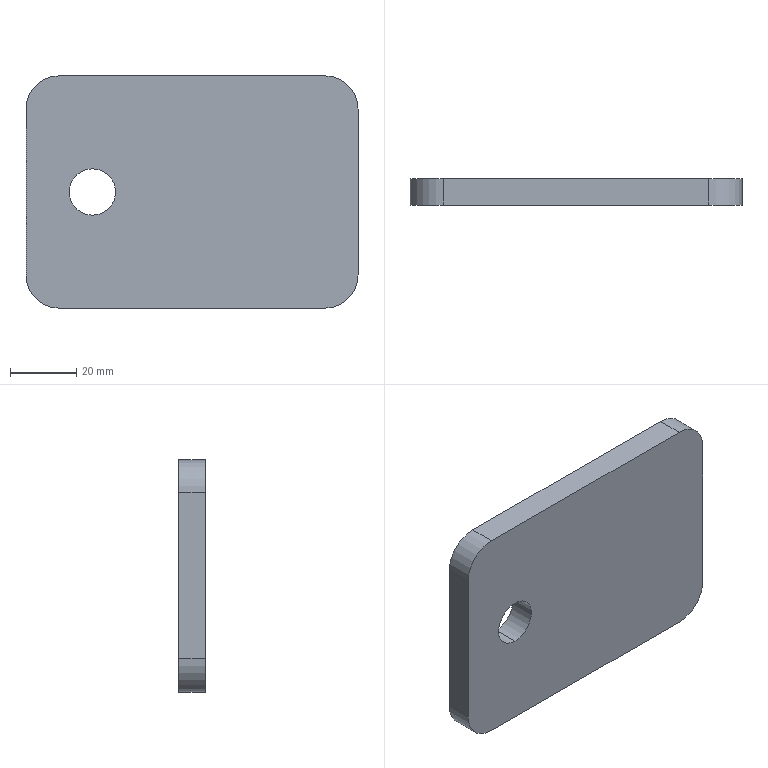Part | SolidWorks | features Extrusion 1, Fillet 1, ICE 1 | 1 solid | 12 faces | box 100 x 8 x 70 mm | volume 54082 mm3 | cylinder 6 | plane 6 | commonest cylinder face diameters 20 x4 14 x2
STEP:
#1=CARTESIAN_POINT('',(-30.,0.,-7.));
#2=VERTEX_POINT('',#1);
#3=CARTESIAN_POINT('',(-30.,0.,7.));
#4=VERTEX_POINT('',#3);
#5=CARTESIAN_POINT('',(-30.,0.,0.));
#6=DIRECTION('',(0.,1.,0.));
#7=DIRECTION('',(0.,0.,1.));
#8=AXIS2_PLACEMENT_3D('',#5,#6,#7);
#9=CIRCLE('',#8,7.);
#10=EDGE_CURVE('',#2,#4,#9,.T.);
#11=ORIENTED_EDGE('',*,*,#10,.F.);
#12=CARTESIAN_POINT('',(-30.,8.,-7.));
#13=VERTEX_POINT('',#12);
#14=CARTESIAN_POINT('',(-30.,0.,-7.));
#15=DIRECTION('',(0.,1.,0.));
#16=VECTOR('',#15,1000.);
#17=LINE('',#14,#16);
#18=EDGE_CURVE('',#2,#13,#17,.T.);
#19=ORIENTED_EDGE('',*,*,#18,.T.);
#20=CARTESIAN_POINT('',(-30.,8.,7.));
#21=VERTEX_POINT('',#20);
#22=CARTESIAN_POINT('',(-30.,8.,0.));
#23=DIRECTION('',(0.,1.,0.));
#24=DIRECTION('',(0.,0.,1.));
#25=AXIS2_PLACEMENT_3D('',#22,#23,#24);
#26=CIRCLE('',#25,7.);
#27=EDGE_CURVE('',#13,#21,#26,.T.);
#28=ORIENTED_EDGE('',*,*,#27,.T.);
#29=CARTESIAN_POINT('',(-30.,0.,7.));
#30=DIRECTION('',(0.,1.,0.));
#31=VECTOR('',#30,1000.);
#32=LINE('',#29,#31);
#33=EDGE_CURVE('',#4,#21,#32,.T.);
#34=ORIENTED_EDGE('',*,*,#33,.F.);
#35=EDGE_LOOP('',(#11,#19,#28,#34));
#36=FACE_OUTER_BOUND('',#35,.T.);
#37=CARTESIAN_POINT('',(-30.,0.,0.));
#38=DIRECTION('',(0.,1.,0.));
#39=DIRECTION('',(0.,0.,1.));
#40=AXIS2_PLACEMENT_3D('',#37,#38,#39);
#41=CYLINDRICAL_SURFACE('',#40,7.);
#42=ADVANCED_FACE('',(#36),#41,.F.);
#43=CARTESIAN_POINT('',(-50.,8.,-25.));
#44=VERTEX_POINT('',#43);
#45=CARTESIAN_POINT('',(-50.,8.,25.));
#46=VERTEX_POINT('',#45);
#47=CARTESIAN_POINT('',(-50.,8.,35.));
#48=DIRECTION('',(0.,0.,1.));
#49=VECTOR('',#48,1000.);
#50=LINE('',#47,#49);
#51=EDGE_CURVE('',#44,#46,#50,.T.);
#52=ORIENTED_EDGE('',*,*,#51,.F.);
#53=CARTESIAN_POINT('',(-50.,0.,-25.));
#54=VERTEX_POINT('',#53);
#55=CARTESIAN_POINT('',(-50.,8.,-25.));
#56=DIRECTION('',(0.,-1.,0.));
#57=VECTOR('',#56,1000.);
#58=LINE('',#55,#57);
#59=EDGE_CURVE('',#44,#54,#58,.T.);
#60=ORIENTED_EDGE('',*,*,#59,.T.);
#61=CARTESIAN_POINT('',(-50.,0.,25.));
#62=VERTEX_POINT('',#61);
#63=CARTESIAN_POINT('',(-50.,0.,35.));
#64=DIRECTION('',(0.,0.,1.));
#65=VECTOR('',#64,1000.);
#66=LINE('',#63,#65);
#67=EDGE_CURVE('',#54,#62,#66,.T.);
#68=ORIENTED_EDGE('',*,*,#67,.T.);
#69=CARTESIAN_POINT('',(-50.,8.,25.));
#70=DIRECTION('',(0.,1.,0.));
#71=VECTOR('',#70,1000.);
#72=LINE('',#69,#71);
#73=EDGE_CURVE('',#62,#46,#72,.T.);
#74=ORIENTED_EDGE('',*,*,#73,.T.);
#75=EDGE_LOOP('',(#52,#60,#68,#74));
#76=FACE_OUTER_BOUND('',#75,.T.);
#77=CARTESIAN_POINT('',(-50.,8.,35.));
#78=DIRECTION('',(1.,0.,0.));
#79=DIRECTION('',(0.,0.,-1.));
#80=AXIS2_PLACEMENT_3D('',#77,#78,#79);
#81=PLANE('',#80);
#82=ADVANCED_FACE('',(#76),#81,.F.);
#83=CARTESIAN_POINT('',(-40.,0.,35.));
#84=VERTEX_POINT('',#83);
#85=CARTESIAN_POINT('',(40.,0.,35.));
#86=VERTEX_POINT('',#85);
#87=CARTESIAN_POINT('',(50.,0.,35.));
#88=DIRECTION('',(1.,0.,0.));
#89=VECTOR('',#88,1000.);
#90=LINE('',#87,#89);
#91=EDGE_CURVE('',#84,#86,#90,.T.);
#92=ORIENTED_EDGE('',*,*,#91,.T.);
#93=CARTESIAN_POINT('',(40.,8.,35.));
#94=VERTEX_POINT('',#93);
#95=CARTESIAN_POINT('',(40.,8.,35.));
#96=DIRECTION('',(0.,1.,0.));
#97=VECTOR('',#96,1000.);
#98=LINE('',#95,#97);
#99=EDGE_CURVE('',#86,#94,#98,.T.);
#100=ORIENTED_EDGE('',*,*,#99,.T.);
#101=CARTESIAN_POINT('',(-40.,8.,35.));
#102=VERTEX_POINT('',#101);
#103=CARTESIAN_POINT('',(50.,8.,35.));
#104=DIRECTION('',(1.,0.,0.));
#105=VECTOR('',#104,1000.);
#106=LINE('',#103,#105);
#107=EDGE_CURVE('',#102,#94,#106,.T.);
#108=ORIENTED_EDGE('',*,*,#107,.F.);
#109=CARTESIAN_POINT('',(-40.,8.,35.));
#110=DIRECTION('',(0.,-1.,0.));
#111=VECTOR('',#110,1000.);
#112=LINE('',#109,#111);
#113=EDGE_CURVE('',#102,#84,#112,.T.);
#114=ORIENTED_EDGE('',*,*,#113,.T.);
#115=EDGE_LOOP('',(#92,#100,#108,#114));
#116=FACE_OUTER_BOUND('',#115,.T.);
#117=CARTESIAN_POINT('',(50.,8.,35.));
#118=DIRECTION('',(0.,0.,-1.));
#119=DIRECTION('',(-1.,0.,0.));
#120=AXIS2_PLACEMENT_3D('',#117,#118,#119);
#121=PLANE('',#120);
#122=ADVANCED_FACE('',(#116),#121,.F.);
#123=CARTESIAN_POINT('',(50.,0.,25.));
#124=VERTEX_POINT('',#123);
#125=CARTESIAN_POINT('',(50.,0.,-25.));
#126=VERTEX_POINT('',#125);
#127=CARTESIAN_POINT('',(50.,0.,35.));
#128=DIRECTION('',(0.,0.,-1.));
#129=VECTOR('',#128,1000.);
#130=LINE('',#127,#129);
#131=EDGE_CURVE('',#124,#126,#130,.T.);
#132=ORIENTED_EDGE('',*,*,#131,.T.);
#133=CARTESIAN_POINT('',(50.,8.,-25.));
#134=VERTEX_POINT('',#133);
#135=CARTESIAN_POINT('',(50.,8.,-25.));
#136=DIRECTION('',(0.,1.,0.));
#137=VECTOR('',#136,1000.);
#138=LINE('',#135,#137);
#139=EDGE_CURVE('',#126,#134,#138,.T.);
#140=ORIENTED_EDGE('',*,*,#139,.T.);
#141=CARTESIAN_POINT('',(50.,8.,25.));
#142=VERTEX_POINT('',#141);
#143=CARTESIAN_POINT('',(50.,8.,35.));
#144=DIRECTION('',(0.,0.,-1.));
#145=VECTOR('',#144,1000.);
#146=LINE('',#143,#145);
#147=EDGE_CURVE('',#142,#134,#146,.T.);
#148=ORIENTED_EDGE('',*,*,#147,.F.);
#149=CARTESIAN_POINT('',(50.,8.,25.));
#150=DIRECTION('',(0.,-1.,0.));
#151=VECTOR('',#150,1000.);
#152=LINE('',#149,#151);
#153=EDGE_CURVE('',#142,#124,#152,.T.);
#154=ORIENTED_EDGE('',*,*,#153,.T.);
#155=EDGE_LOOP('',(#132,#140,#148,#154));
#156=FACE_OUTER_BOUND('',#155,.T.);
#157=CARTESIAN_POINT('',(50.,8.,35.));
#158=DIRECTION('',(-1.,0.,0.));
#159=DIRECTION('',(0.,0.,1.));
#160=AXIS2_PLACEMENT_3D('',#157,#158,#159);
#161=PLANE('',#160);
#162=ADVANCED_FACE('',(#156),#161,.F.);
#163=CARTESIAN_POINT('',(40.,0.,-35.));
#164=VERTEX_POINT('',#163);
#165=CARTESIAN_POINT('',(-40.,0.,-35.));
#166=VERTEX_POINT('',#165);
#167=CARTESIAN_POINT('',(50.,0.,-35.));
#168=DIRECTION('',(-1.,0.,0.));
#169=VECTOR('',#168,1000.);
#170=LINE('',#167,#169);
#171=EDGE_CURVE('',#164,#166,#170,.T.);
#172=ORIENTED_EDGE('',*,*,#171,.T.);
#173=CARTESIAN_POINT('',(-40.,8.,-35.));
#174=VERTEX_POINT('',#173);
#175=CARTESIAN_POINT('',(-40.,8.,-35.));
#176=DIRECTION('',(0.,1.,0.));
#177=VECTOR('',#176,1000.);
#178=LINE('',#175,#177);
#179=EDGE_CURVE('',#166,#174,#178,.T.);
#180=ORIENTED_EDGE('',*,*,#179,.T.);
#181=CARTESIAN_POINT('',(40.,8.,-35.));
#182=VERTEX_POINT('',#181);
#183=CARTESIAN_POINT('',(50.,8.,-35.));
#184=DIRECTION('',(-1.,0.,0.));
#185=VECTOR('',#184,1000.);
#186=LINE('',#183,#185);
#187=EDGE_CURVE('',#182,#174,#186,.T.);
#188=ORIENTED_EDGE('',*,*,#187,.F.);
#189=CARTESIAN_POINT('',(40.,8.,-35.));
#190=DIRECTION('',(0.,-1.,0.));
#191=VECTOR('',#190,1000.);
#192=LINE('',#189,#191);
#193=EDGE_CURVE('',#182,#164,#192,.T.);
#194=ORIENTED_EDGE('',*,*,#193,.T.);
#195=EDGE_LOOP('',(#172,#180,#188,#194));
#196=FACE_OUTER_BOUND('',#195,.T.);
#197=CARTESIAN_POINT('',(50.,8.,-35.));
#198=DIRECTION('',(0.,0.,1.));
#199=DIRECTION('',(1.,0.,0.));
#200=AXIS2_PLACEMENT_3D('',#197,#198,#199);
#201=PLANE('',#200);
#202=ADVANCED_FACE('',(#196),#201,.F.);
#203=CARTESIAN_POINT('',(-30.,8.,0.));
#204=DIRECTION('',(0.,1.,0.));
#205=DIRECTION('',(0.,0.,1.));
#206=AXIS2_PLACEMENT_3D('',#203,#204,#205);
#207=CIRCLE('',#206,7.);
#208=EDGE_CURVE('',#21,#13,#207,.T.);
#209=ORIENTED_EDGE('',*,*,#208,.F.);
#210=ORIENTED_EDGE('',*,*,#27,.F.);
#211=EDGE_LOOP('',(#209,#210));
#212=FACE_BOUND('',#211,.T.);
#213=ORIENTED_EDGE('',*,*,#187,.T.);
#214=CARTESIAN_POINT('',(-40.,8.,-25.));
#215=DIRECTION('',(0.,1.,0.));
#216=DIRECTION('',(0.,0.,1.));
#217=AXIS2_PLACEMENT_3D('',#214,#215,#216);
#218=CIRCLE('',#217,10.);
#219=EDGE_CURVE('',#174,#44,#218,.T.);
#220=ORIENTED_EDGE('',*,*,#219,.T.);
#221=ORIENTED_EDGE('',*,*,#51,.T.);
#222=CARTESIAN_POINT('',(-40.,8.,25.));
#223=DIRECTION('',(0.,1.,0.));
#224=DIRECTION('',(0.,0.,1.));
#225=AXIS2_PLACEMENT_3D('',#222,#223,#224);
#226=CIRCLE('',#225,10.);
#227=EDGE_CURVE('',#46,#102,#226,.T.);
#228=ORIENTED_EDGE('',*,*,#227,.T.);
#229=ORIENTED_EDGE('',*,*,#107,.T.);
#230=CARTESIAN_POINT('',(40.,8.,25.));
#231=DIRECTION('',(0.,1.,0.));
#232=DIRECTION('',(0.,0.,1.));
#233=AXIS2_PLACEMENT_3D('',#230,#231,#232);
#234=CIRCLE('',#233,10.);
#235=EDGE_CURVE('',#94,#142,#234,.T.);
#236=ORIENTED_EDGE('',*,*,#235,.T.);
#237=ORIENTED_EDGE('',*,*,#147,.T.);
#238=CARTESIAN_POINT('',(40.,8.,-25.));
#239=DIRECTION('',(0.,1.,0.));
#240=DIRECTION('',(0.,0.,1.));
#241=AXIS2_PLACEMENT_3D('',#238,#239,#240);
#242=CIRCLE('',#241,10.);
#243=EDGE_CURVE('',#134,#182,#242,.T.);
#244=ORIENTED_EDGE('',*,*,#243,.T.);
#245=EDGE_LOOP('',(#213,#220,#221,#228,#229,#236,#237,#244));
#246=FACE_OUTER_BOUND('',#245,.T.);
#247=CARTESIAN_POINT('',(0.,8.,0.));
#248=DIRECTION('',(0.,1.,0.));
#249=DIRECTION('',(0.,0.,1.));
#250=AXIS2_PLACEMENT_3D('',#247,#248,#249);
#251=PLANE('',#250);
#252=ADVANCED_FACE('',(#212,#246),#251,.T.);
#253=CARTESIAN_POINT('',(-30.,0.,0.));
#254=DIRECTION('',(0.,1.,0.));
#255=DIRECTION('',(0.,0.,1.));
#256=AXIS2_PLACEMENT_3D('',#253,#254,#255);
#257=CIRCLE('',#256,7.);
#258=EDGE_CURVE('',#4,#2,#257,.T.);
#259=ORIENTED_EDGE('',*,*,#258,.T.);
#260=ORIENTED_EDGE('',*,*,#10,.T.);
#261=EDGE_LOOP('',(#259,#260));
#262=FACE_BOUND('',#261,.T.);
#263=ORIENTED_EDGE('',*,*,#67,.F.);
#264=CARTESIAN_POINT('',(-40.,0.,-25.));
#265=DIRECTION('',(0.,-1.,0.));
#266=DIRECTION('',(0.,0.,1.));
#267=AXIS2_PLACEMENT_3D('',#264,#265,#266);
#268=CIRCLE('',#267,10.);
#269=EDGE_CURVE('',#54,#166,#268,.T.);
#270=ORIENTED_EDGE('',*,*,#269,.T.);
#271=ORIENTED_EDGE('',*,*,#171,.F.);
#272=CARTESIAN_POINT('',(40.,0.,-25.));
#273=DIRECTION('',(0.,-1.,0.));
#274=DIRECTION('',(0.,0.,1.));
#275=AXIS2_PLACEMENT_3D('',#272,#273,#274);
#276=CIRCLE('',#275,10.);
#277=EDGE_CURVE('',#164,#126,#276,.T.);
#278=ORIENTED_EDGE('',*,*,#277,.T.);
#279=ORIENTED_EDGE('',*,*,#131,.F.);
#280=CARTESIAN_POINT('',(40.,0.,25.));
#281=DIRECTION('',(0.,-1.,0.));
#282=DIRECTION('',(0.,0.,1.));
#283=AXIS2_PLACEMENT_3D('',#280,#281,#282);
#284=CIRCLE('',#283,10.);
#285=EDGE_CURVE('',#124,#86,#284,.T.);
#286=ORIENTED_EDGE('',*,*,#285,.T.);
#287=ORIENTED_EDGE('',*,*,#91,.F.);
#288=CARTESIAN_POINT('',(-40.,0.,25.));
#289=DIRECTION('',(0.,-1.,0.));
#290=DIRECTION('',(0.,0.,1.));
#291=AXIS2_PLACEMENT_3D('',#288,#289,#290);
#292=CIRCLE('',#291,10.);
#293=EDGE_CURVE('',#84,#62,#292,.T.);
#294=ORIENTED_EDGE('',*,*,#293,.T.);
#295=EDGE_LOOP('',(#263,#270,#271,#278,#279,#286,#287,#294));
#296=FACE_OUTER_BOUND('',#295,.T.);
#297=CARTESIAN_POINT('',(0.,0.,0.));
#298=DIRECTION('',(0.,1.,0.));
#299=DIRECTION('',(0.,0.,1.));
#300=AXIS2_PLACEMENT_3D('',#297,#298,#299);
#301=PLANE('',#300);
#302=ADVANCED_FACE('',(#262,#296),#301,.F.);
#303=ORIENTED_EDGE('',*,*,#219,.F.);
#304=ORIENTED_EDGE('',*,*,#179,.F.);
#305=ORIENTED_EDGE('',*,*,#269,.F.);
#306=ORIENTED_EDGE('',*,*,#59,.F.);
#307=EDGE_LOOP('',(#303,#304,#305,#306));
#308=FACE_OUTER_BOUND('',#307,.T.);
#309=CARTESIAN_POINT('',(-40.,8.,-25.));
#310=DIRECTION('',(0.,-1.,0.));
#311=DIRECTION('',(0.,0.,-1.));
#312=AXIS2_PLACEMENT_3D('',#309,#310,#311);
#313=CYLINDRICAL_SURFACE('',#312,10.);
#314=ADVANCED_FACE('',(#308),#313,.T.);
#315=ORIENTED_EDGE('',*,*,#243,.F.);
#316=ORIENTED_EDGE('',*,*,#139,.F.);
#317=ORIENTED_EDGE('',*,*,#277,.F.);
#318=ORIENTED_EDGE('',*,*,#193,.F.);
#319=EDGE_LOOP('',(#315,#316,#317,#318));
#320=FACE_OUTER_BOUND('',#319,.T.);
#321=CARTESIAN_POINT('',(40.,8.,-25.));
#322=DIRECTION('',(0.,-1.,0.));
#323=DIRECTION('',(0.,0.,-1.));
#324=AXIS2_PLACEMENT_3D('',#321,#322,#323);
#325=CYLINDRICAL_SURFACE('',#324,10.);
#326=ADVANCED_FACE('',(#320),#325,.T.);
#327=ORIENTED_EDGE('',*,*,#235,.F.);
#328=ORIENTED_EDGE('',*,*,#99,.F.);
#329=ORIENTED_EDGE('',*,*,#285,.F.);
#330=ORIENTED_EDGE('',*,*,#153,.F.);
#331=EDGE_LOOP('',(#327,#328,#329,#330));
#332=FACE_OUTER_BOUND('',#331,.T.);
#333=CARTESIAN_POINT('',(40.,8.,25.));
#334=DIRECTION('',(0.,-1.,0.));
#335=DIRECTION('',(0.,0.,-1.));
#336=AXIS2_PLACEMENT_3D('',#333,#334,#335);
#337=CYLINDRICAL_SURFACE('',#336,10.);
#338=ADVANCED_FACE('',(#332),#337,.T.);
#339=ORIENTED_EDGE('',*,*,#227,.F.);
#340=ORIENTED_EDGE('',*,*,#73,.F.);
#341=ORIENTED_EDGE('',*,*,#293,.F.);
#342=ORIENTED_EDGE('',*,*,#113,.F.);
#343=EDGE_LOOP('',(#339,#340,#341,#342));
#344=FACE_OUTER_BOUND('',#343,.T.);
#345=CARTESIAN_POINT('',(-40.,8.,25.));
#346=DIRECTION('',(0.,-1.,0.));
#347=DIRECTION('',(0.,0.,-1.));
#348=AXIS2_PLACEMENT_3D('',#345,#346,#347);
#349=CYLINDRICAL_SURFACE('',#348,10.);
#350=ADVANCED_FACE('',(#344),#349,.T.);
#351=ORIENTED_EDGE('',*,*,#18,.F.);
#352=ORIENTED_EDGE('',*,*,#258,.F.);
#353=ORIENTED_EDGE('',*,*,#33,.T.);
#354=ORIENTED_EDGE('',*,*,#208,.T.);
#355=EDGE_LOOP('',(#351,#352,#353,#354));
#356=FACE_OUTER_BOUND('',#355,.T.);
#357=CARTESIAN_POINT('',(-30.,0.,0.));
#358=DIRECTION('',(0.,1.,0.));
#359=DIRECTION('',(0.,0.,1.));
#360=AXIS2_PLACEMENT_3D('',#357,#358,#359);
#361=CYLINDRICAL_SURFACE('',#360,7.);
#362=ADVANCED_FACE('',(#356),#361,.F.);
#363=CLOSED_SHELL('',(#42,#82,#122,#162,#202,#252,#302,#314,#326,#338,#350,#362));
#364=MANIFOLD_SOLID_BREP('',#363);
#365=CARTESIAN_POINT('',(0.,0.,0.));
#366=DIRECTION('',(0.,0.,1.));
#367=DIRECTION('',(1.,0.,0.));
#368=AXIS2_PLACEMENT_3D('',#365,#366,#367);
#369=(LENGTH_UNIT()NAMED_UNIT(*)SI_UNIT(.MILLI.,.METRE.));
#370=UNCERTAINTY_MEASURE_WITH_UNIT(LENGTH_MEASURE(0.00001),#369,'','');
#371=(NAMED_UNIT(*)PLANE_ANGLE_UNIT()SI_UNIT($,.RADIAN.));
#372=(NAMED_UNIT(*)SI_UNIT($,.STERADIAN.)SOLID_ANGLE_UNIT());
#373=(GEOMETRIC_REPRESENTATION_CONTEXT(3)GLOBAL_UNCERTAINTY_ASSIGNED_CONTEXT((#370))GLOBAL_UNIT_ASSIGNED_CONTEXT((#369,#371,#372))REPRESENTATION_CONTEXT('',''));
#374=ADVANCED_BREP_SHAPE_REPRESENTATION('',(#364,#368),#373);